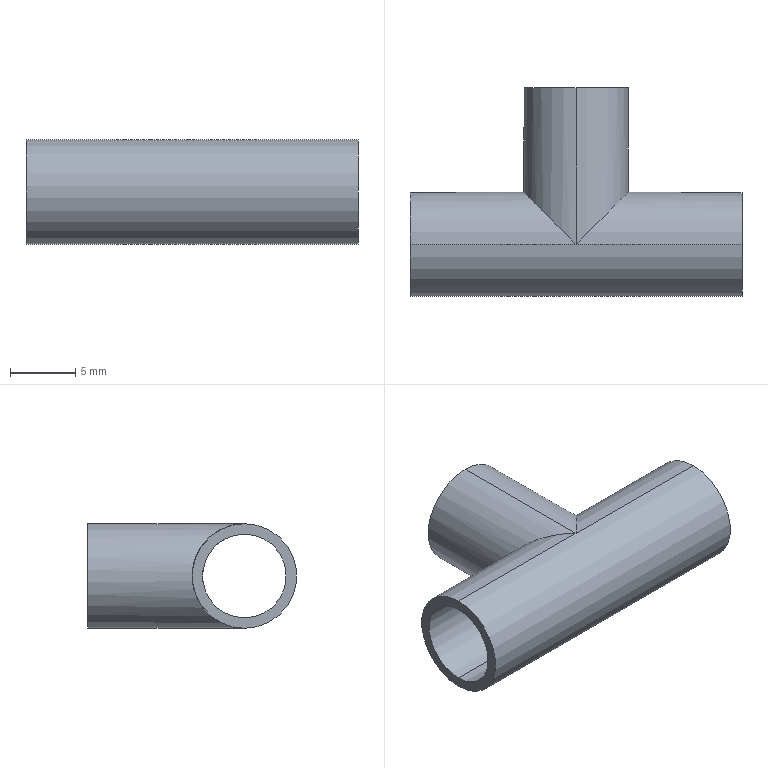Part | STEP file | quarter tee_default_machined_ | 2 solids | 15 faces | box 25.4 x 16 x 8 mm | volume 593.284 mm3 | cylinder 12 | plane 3 | commonest cylinder face diameters 6.4 x7 8 x5